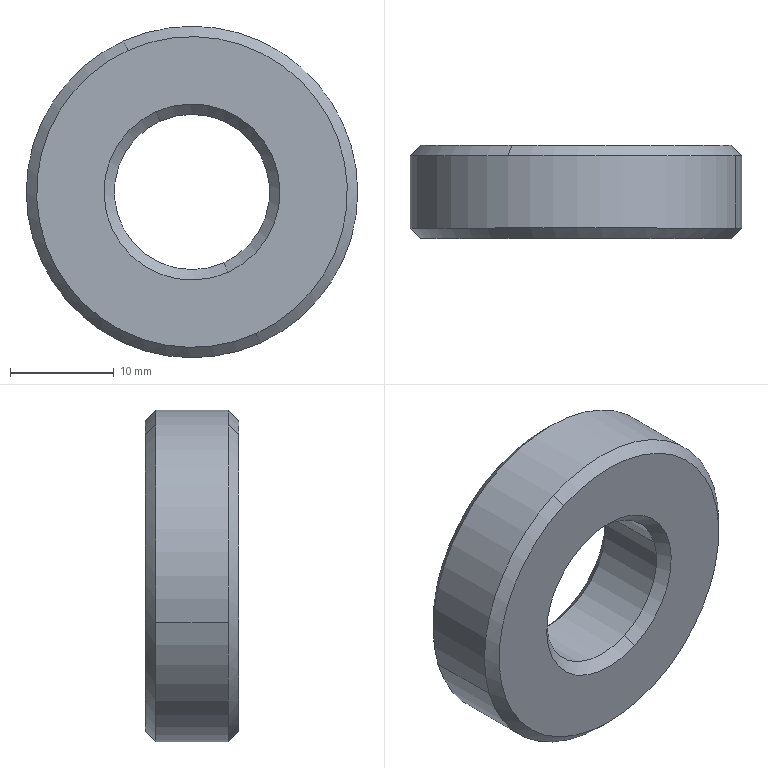Part | SolidWorks | features BaseBody 1 | 1 solid | 14 faces | box 32 x 9 x 32 mm | volume 5500 mm3 | cone 8 | cylinder 4 | plane 2 | commonest cylinder face diameters 15 x2 32 x2
STEP:
#1=CARTESIAN_POINT('',(-381.352,-113.,29.799));
#2=VERTEX_POINT('',#1);
#3=CARTESIAN_POINT('',(-393.697,-113.,57.141));
#4=VERTEX_POINT('',#3);
#5=CARTESIAN_POINT('',(-387.524,-113.,43.47));
#6=DIRECTION('',(0.,1.,0.));
#7=DIRECTION('',(-0.9598,0.,-0.2807));
#8=AXIS2_PLACEMENT_3D('',#5,#6,#7);
#9=CIRCLE('',#8,15.);
#10=EDGE_CURVE('',#2,#4,#9,.T.);
#11=ORIENTED_EDGE('',*,*,#10,.F.);
#12=CARTESIAN_POINT('',(-380.94,-114.,28.888));
#13=VERTEX_POINT('',#12);
#14=CARTESIAN_POINT('',(-381.146,-113.5,29.343));
#15=DIRECTION('',(0.291,-0.7071,-0.6445));
#16=VECTOR('',#15,1000.);
#17=LINE('',#14,#16);
#18=EDGE_CURVE('',#2,#13,#17,.T.);
#19=ORIENTED_EDGE('',*,*,#18,.T.);
#20=CARTESIAN_POINT('',(-402.881,-114.,38.979));
#21=VERTEX_POINT('',#20);
#22=CARTESIAN_POINT('',(-387.524,-114.,43.47));
#23=DIRECTION('',(0.,1.,0.));
#24=DIRECTION('',(-0.9598,0.,-0.2807));
#25=AXIS2_PLACEMENT_3D('',#22,#23,#24);
#26=CIRCLE('',#25,16.);
#27=EDGE_CURVE('',#13,#21,#26,.T.);
#28=ORIENTED_EDGE('',*,*,#27,.T.);
#29=CARTESIAN_POINT('',(-394.109,-114.,58.053));
#30=VERTEX_POINT('',#29);
#31=CARTESIAN_POINT('',(-387.524,-114.,43.47));
#32=DIRECTION('',(0.,1.,0.));
#33=DIRECTION('',(-0.9598,0.,-0.2807));
#34=AXIS2_PLACEMENT_3D('',#31,#32,#33);
#35=CIRCLE('',#34,16.);
#36=EDGE_CURVE('',#21,#30,#35,.T.);
#37=ORIENTED_EDGE('',*,*,#36,.T.);
#38=CARTESIAN_POINT('',(-393.903,-113.5,57.597));
#39=DIRECTION('',(-0.291,-0.7071,0.6445));
#40=VECTOR('',#39,1000.);
#41=LINE('',#38,#40);
#42=EDGE_CURVE('',#4,#30,#41,.T.);
#43=ORIENTED_EDGE('',*,*,#42,.F.);
#44=EDGE_LOOP('',(#11,#19,#28,#37,#43));
#45=FACE_OUTER_BOUND('',#44,.T.);
#46=CARTESIAN_POINT('',(-387.524,-113.5,43.47));
#47=DIRECTION('',(0.,-1.,0.));
#48=DIRECTION('',(-0.4115,0.,0.9114));
#49=AXIS2_PLACEMENT_3D('',#46,#47,#48);
#50=CONICAL_SURFACE('',#49,15.5,0.7854);
#51=ADVANCED_FACE('',(#45),#50,.T.);
#52=CARTESIAN_POINT('',(-381.352,-122.,29.799));
#53=VERTEX_POINT('',#52);
#54=CARTESIAN_POINT('',(-393.697,-122.,57.141));
#55=VERTEX_POINT('',#54);
#56=CARTESIAN_POINT('',(-387.524,-122.,43.47));
#57=DIRECTION('',(0.,-1.,0.));
#58=DIRECTION('',(0.9598,0.,0.2807));
#59=AXIS2_PLACEMENT_3D('',#56,#57,#58);
#60=CIRCLE('',#59,15.);
#61=EDGE_CURVE('',#53,#55,#60,.T.);
#62=ORIENTED_EDGE('',*,*,#61,.F.);
#63=CARTESIAN_POINT('',(-380.94,-121.,28.888));
#64=VERTEX_POINT('',#63);
#65=CARTESIAN_POINT('',(-381.146,-121.5,29.343));
#66=DIRECTION('',(0.291,0.7071,-0.6445));
#67=VECTOR('',#66,1000.);
#68=LINE('',#65,#67);
#69=EDGE_CURVE('',#53,#64,#68,.T.);
#70=ORIENTED_EDGE('',*,*,#69,.T.);
#71=CARTESIAN_POINT('',(-372.168,-121.,47.961));
#72=VERTEX_POINT('',#71);
#73=CARTESIAN_POINT('',(-387.524,-121.,43.47));
#74=DIRECTION('',(0.,-1.,0.));
#75=DIRECTION('',(0.9598,0.,0.2807));
#76=AXIS2_PLACEMENT_3D('',#73,#74,#75);
#77=CIRCLE('',#76,16.);
#78=EDGE_CURVE('',#64,#72,#77,.T.);
#79=ORIENTED_EDGE('',*,*,#78,.T.);
#80=CARTESIAN_POINT('',(-394.109,-121.,58.053));
#81=VERTEX_POINT('',#80);
#82=CARTESIAN_POINT('',(-387.524,-121.,43.47));
#83=DIRECTION('',(0.,-1.,0.));
#84=DIRECTION('',(0.9598,0.,0.2807));
#85=AXIS2_PLACEMENT_3D('',#82,#83,#84);
#86=CIRCLE('',#85,16.);
#87=EDGE_CURVE('',#72,#81,#86,.T.);
#88=ORIENTED_EDGE('',*,*,#87,.T.);
#89=CARTESIAN_POINT('',(-393.903,-121.5,57.597));
#90=DIRECTION('',(-0.291,0.7071,0.6445));
#91=VECTOR('',#90,1000.);
#92=LINE('',#89,#91);
#93=EDGE_CURVE('',#55,#81,#92,.T.);
#94=ORIENTED_EDGE('',*,*,#93,.F.);
#95=EDGE_LOOP('',(#62,#70,#79,#88,#94));
#96=FACE_OUTER_BOUND('',#95,.T.);
#97=CARTESIAN_POINT('',(-387.524,-121.5,43.47));
#98=DIRECTION('',(0.,1.,0.));
#99=DIRECTION('',(-0.4115,0.,0.9114));
#100=AXIS2_PLACEMENT_3D('',#97,#98,#99);
#101=CONICAL_SURFACE('',#100,15.5,0.7854);
#102=ADVANCED_FACE('',(#96),#101,.T.);
#103=CARTESIAN_POINT('',(-380.326,-121.,45.575));
#104=VERTEX_POINT('',#103);
#105=CARTESIAN_POINT('',(-384.438,-121.,36.635));
#106=VERTEX_POINT('',#105);
#107=CARTESIAN_POINT('',(-387.524,-121.,43.47));
#108=DIRECTION('',(0.,1.,0.));
#109=DIRECTION('',(-0.9598,0.,-0.2807));
#110=AXIS2_PLACEMENT_3D('',#107,#108,#109);
#111=CIRCLE('',#110,7.5);
#112=EDGE_CURVE('',#104,#106,#111,.T.);
#113=ORIENTED_EDGE('',*,*,#112,.T.);
#114=CARTESIAN_POINT('',(-384.027,-122.,35.723));
#115=VERTEX_POINT('',#114);
#116=CARTESIAN_POINT('',(-384.232,-121.5,36.179));
#117=DIRECTION('',(0.291,-0.7071,-0.6445));
#118=VECTOR('',#117,1000.);
#119=LINE('',#116,#118);
#120=EDGE_CURVE('',#106,#115,#119,.T.);
#121=ORIENTED_EDGE('',*,*,#120,.T.);
#122=CARTESIAN_POINT('',(-391.022,-122.,51.217));
#123=VERTEX_POINT('',#122);
#124=CARTESIAN_POINT('',(-387.524,-122.,43.47));
#125=DIRECTION('',(0.,1.,0.));
#126=DIRECTION('',(-0.9598,0.,-0.2807));
#127=AXIS2_PLACEMENT_3D('',#124,#125,#126);
#128=CIRCLE('',#127,8.5);
#129=EDGE_CURVE('',#123,#115,#128,.T.);
#130=ORIENTED_EDGE('',*,*,#129,.F.);
#131=CARTESIAN_POINT('',(-390.611,-121.,50.306));
#132=VERTEX_POINT('',#131);
#133=CARTESIAN_POINT('',(-390.817,-121.5,50.761));
#134=DIRECTION('',(-0.291,-0.7071,0.6445));
#135=VECTOR('',#134,1000.);
#136=LINE('',#133,#135);
#137=EDGE_CURVE('',#132,#123,#136,.T.);
#138=ORIENTED_EDGE('',*,*,#137,.F.);
#139=CARTESIAN_POINT('',(-387.524,-121.,43.47));
#140=DIRECTION('',(0.,1.,0.));
#141=DIRECTION('',(-0.9598,0.,-0.2807));
#142=AXIS2_PLACEMENT_3D('',#139,#140,#141);
#143=CIRCLE('',#142,7.5);
#144=EDGE_CURVE('',#132,#104,#143,.T.);
#145=ORIENTED_EDGE('',*,*,#144,.T.);
#146=EDGE_LOOP('',(#113,#121,#130,#138,#145));
#147=FACE_OUTER_BOUND('',#146,.T.);
#148=CARTESIAN_POINT('',(-387.524,-121.5,43.47));
#149=DIRECTION('',(0.,-1.,0.));
#150=DIRECTION('',(-0.4115,0.,0.9114));
#151=AXIS2_PLACEMENT_3D('',#148,#149,#150);
#152=CONICAL_SURFACE('',#151,8.,0.7854);
#153=ADVANCED_FACE('',(#147),#152,.F.);
#154=CARTESIAN_POINT('',(-394.723,-114.,41.365));
#155=VERTEX_POINT('',#154);
#156=CARTESIAN_POINT('',(-384.438,-114.,36.635));
#157=VERTEX_POINT('',#156);
#158=CARTESIAN_POINT('',(-387.524,-114.,43.47));
#159=DIRECTION('',(0.,-1.,0.));
#160=DIRECTION('',(0.9598,0.,0.2807));
#161=AXIS2_PLACEMENT_3D('',#158,#159,#160);
#162=CIRCLE('',#161,7.5);
#163=EDGE_CURVE('',#155,#157,#162,.T.);
#164=ORIENTED_EDGE('',*,*,#163,.T.);
#165=CARTESIAN_POINT('',(-384.027,-113.,35.723));
#166=VERTEX_POINT('',#165);
#167=CARTESIAN_POINT('',(-384.232,-113.5,36.179));
#168=DIRECTION('',(0.291,0.7071,-0.6445));
#169=VECTOR('',#168,1000.);
#170=LINE('',#167,#169);
#171=EDGE_CURVE('',#157,#166,#170,.T.);
#172=ORIENTED_EDGE('',*,*,#171,.T.);
#173=CARTESIAN_POINT('',(-391.022,-113.,51.217));
#174=VERTEX_POINT('',#173);
#175=CARTESIAN_POINT('',(-387.524,-113.,43.47));
#176=DIRECTION('',(0.,-1.,0.));
#177=DIRECTION('',(0.9598,0.,0.2807));
#178=AXIS2_PLACEMENT_3D('',#175,#176,#177);
#179=CIRCLE('',#178,8.5);
#180=EDGE_CURVE('',#174,#166,#179,.T.);
#181=ORIENTED_EDGE('',*,*,#180,.F.);
#182=CARTESIAN_POINT('',(-390.611,-114.,50.306));
#183=VERTEX_POINT('',#182);
#184=CARTESIAN_POINT('',(-390.817,-113.5,50.761));
#185=DIRECTION('',(-0.291,0.7071,0.6445));
#186=VECTOR('',#185,1000.);
#187=LINE('',#184,#186);
#188=EDGE_CURVE('',#183,#174,#187,.T.);
#189=ORIENTED_EDGE('',*,*,#188,.F.);
#190=CARTESIAN_POINT('',(-387.524,-114.,43.47));
#191=DIRECTION('',(0.,-1.,0.));
#192=DIRECTION('',(0.9598,0.,0.2807));
#193=AXIS2_PLACEMENT_3D('',#190,#191,#192);
#194=CIRCLE('',#193,7.5);
#195=EDGE_CURVE('',#183,#155,#194,.T.);
#196=ORIENTED_EDGE('',*,*,#195,.T.);
#197=EDGE_LOOP('',(#164,#172,#181,#189,#196));
#198=FACE_OUTER_BOUND('',#197,.T.);
#199=CARTESIAN_POINT('',(-387.524,-113.5,43.47));
#200=DIRECTION('',(0.,1.,0.));
#201=DIRECTION('',(-0.4115,0.,0.9114));
#202=AXIS2_PLACEMENT_3D('',#199,#200,#201);
#203=CONICAL_SURFACE('',#202,8.,0.7854);
#204=ADVANCED_FACE('',(#198),#203,.F.);
#205=ORIENTED_EDGE('',*,*,#163,.F.);
#206=CARTESIAN_POINT('',(-394.723,-121.,41.365));
#207=VERTEX_POINT('',#206);
#208=CARTESIAN_POINT('',(-394.723,-113.,41.365));
#209=DIRECTION('',(0.,-1.,0.));
#210=VECTOR('',#209,1000.);
#211=LINE('',#208,#210);
#212=EDGE_CURVE('',#155,#207,#211,.T.);
#213=ORIENTED_EDGE('',*,*,#212,.T.);
#214=CARTESIAN_POINT('',(-387.524,-121.,43.47));
#215=DIRECTION('',(0.,1.,0.));
#216=DIRECTION('',(-0.9598,0.,-0.2807));
#217=AXIS2_PLACEMENT_3D('',#214,#215,#216);
#218=CIRCLE('',#217,7.5);
#219=EDGE_CURVE('',#106,#207,#218,.T.);
#220=ORIENTED_EDGE('',*,*,#219,.F.);
#221=ORIENTED_EDGE('',*,*,#112,.F.);
#222=CARTESIAN_POINT('',(-380.326,-114.,45.575));
#223=VERTEX_POINT('',#222);
#224=CARTESIAN_POINT('',(-380.326,-113.,45.575));
#225=DIRECTION('',(0.,-1.,0.));
#226=VECTOR('',#225,1000.);
#227=LINE('',#224,#226);
#228=EDGE_CURVE('',#223,#104,#227,.T.);
#229=ORIENTED_EDGE('',*,*,#228,.F.);
#230=CARTESIAN_POINT('',(-387.524,-114.,43.47));
#231=DIRECTION('',(0.,-1.,0.));
#232=DIRECTION('',(0.9598,0.,0.2807));
#233=AXIS2_PLACEMENT_3D('',#230,#231,#232);
#234=CIRCLE('',#233,7.5);
#235=EDGE_CURVE('',#157,#223,#234,.T.);
#236=ORIENTED_EDGE('',*,*,#235,.F.);
#237=EDGE_LOOP('',(#205,#213,#220,#221,#229,#236));
#238=FACE_OUTER_BOUND('',#237,.T.);
#239=CARTESIAN_POINT('',(-387.524,-113.,43.47));
#240=DIRECTION('',(0.,-1.,0.));
#241=DIRECTION('',(0.9598,0.,0.2807));
#242=AXIS2_PLACEMENT_3D('',#239,#240,#241);
#243=CYLINDRICAL_SURFACE('',#242,7.5);
#244=ADVANCED_FACE('',(#238),#243,.F.);
#245=ORIENTED_EDGE('',*,*,#36,.F.);
#246=CARTESIAN_POINT('',(-402.881,-121.,38.979));
#247=VERTEX_POINT('',#246);
#248=CARTESIAN_POINT('',(-402.881,-113.,38.979));
#249=DIRECTION('',(0.,-1.,0.));
#250=VECTOR('',#249,1000.);
#251=LINE('',#248,#250);
#252=EDGE_CURVE('',#21,#247,#251,.T.);
#253=ORIENTED_EDGE('',*,*,#252,.T.);
#254=CARTESIAN_POINT('',(-387.524,-121.,43.47));
#255=DIRECTION('',(0.,-1.,0.));
#256=DIRECTION('',(0.9598,0.,0.2807));
#257=AXIS2_PLACEMENT_3D('',#254,#255,#256);
#258=CIRCLE('',#257,16.);
#259=EDGE_CURVE('',#81,#247,#258,.T.);
#260=ORIENTED_EDGE('',*,*,#259,.F.);
#261=ORIENTED_EDGE('',*,*,#87,.F.);
#262=CARTESIAN_POINT('',(-372.168,-114.,47.961));
#263=VERTEX_POINT('',#262);
#264=CARTESIAN_POINT('',(-372.168,-113.,47.961));
#265=DIRECTION('',(0.,-1.,0.));
#266=VECTOR('',#265,1000.);
#267=LINE('',#264,#266);
#268=EDGE_CURVE('',#263,#72,#267,.T.);
#269=ORIENTED_EDGE('',*,*,#268,.F.);
#270=CARTESIAN_POINT('',(-387.524,-114.,43.47));
#271=DIRECTION('',(0.,1.,0.));
#272=DIRECTION('',(-0.9598,0.,-0.2807));
#273=AXIS2_PLACEMENT_3D('',#270,#271,#272);
#274=CIRCLE('',#273,16.);
#275=EDGE_CURVE('',#30,#263,#274,.T.);
#276=ORIENTED_EDGE('',*,*,#275,.F.);
#277=EDGE_LOOP('',(#245,#253,#260,#261,#269,#276));
#278=FACE_OUTER_BOUND('',#277,.T.);
#279=CARTESIAN_POINT('',(-387.524,-113.,43.47));
#280=DIRECTION('',(0.,-1.,0.));
#281=DIRECTION('',(0.9598,0.,0.2807));
#282=AXIS2_PLACEMENT_3D('',#279,#280,#281);
#283=CYLINDRICAL_SURFACE('',#282,16.);
#284=ADVANCED_FACE('',(#278),#283,.T.);
#285=ORIENTED_EDGE('',*,*,#180,.T.);
#286=CARTESIAN_POINT('',(-387.524,-113.,43.47));
#287=DIRECTION('',(0.,-1.,0.));
#288=DIRECTION('',(0.9598,0.,0.2807));
#289=AXIS2_PLACEMENT_3D('',#286,#287,#288);
#290=CIRCLE('',#289,8.5);
#291=EDGE_CURVE('',#166,#174,#290,.T.);
#292=ORIENTED_EDGE('',*,*,#291,.T.);
#293=EDGE_LOOP('',(#285,#292));
#294=FACE_BOUND('',#293,.T.);
#295=CARTESIAN_POINT('',(-387.524,-113.,43.47));
#296=DIRECTION('',(0.,1.,0.));
#297=DIRECTION('',(-0.9598,0.,-0.2807));
#298=AXIS2_PLACEMENT_3D('',#295,#296,#297);
#299=CIRCLE('',#298,15.);
#300=EDGE_CURVE('',#4,#2,#299,.T.);
#301=ORIENTED_EDGE('',*,*,#300,.T.);
#302=ORIENTED_EDGE('',*,*,#10,.T.);
#303=EDGE_LOOP('',(#301,#302));
#304=FACE_OUTER_BOUND('',#303,.T.);
#305=CARTESIAN_POINT('',(-402.493,-113.,22.962));
#306=DIRECTION('',(0.,-1.,0.));
#307=DIRECTION('',(0.,0.,-1.));
#308=AXIS2_PLACEMENT_3D('',#305,#306,#307);
#309=PLANE('',#308);
#310=ADVANCED_FACE('',(#294,#304),#309,.F.);
#311=ORIENTED_EDGE('',*,*,#129,.T.);
#312=CARTESIAN_POINT('',(-387.524,-122.,43.47));
#313=DIRECTION('',(0.,1.,0.));
#314=DIRECTION('',(-0.9598,0.,-0.2807));
#315=AXIS2_PLACEMENT_3D('',#312,#313,#314);
#316=CIRCLE('',#315,8.5);
#317=EDGE_CURVE('',#115,#123,#316,.T.);
#318=ORIENTED_EDGE('',*,*,#317,.T.);
#319=EDGE_LOOP('',(#311,#318));
#320=FACE_BOUND('',#319,.T.);
#321=CARTESIAN_POINT('',(-387.524,-122.,43.47));
#322=DIRECTION('',(0.,-1.,0.));
#323=DIRECTION('',(0.9598,0.,0.2807));
#324=AXIS2_PLACEMENT_3D('',#321,#322,#323);
#325=CIRCLE('',#324,15.);
#326=EDGE_CURVE('',#55,#53,#325,.T.);
#327=ORIENTED_EDGE('',*,*,#326,.T.);
#328=ORIENTED_EDGE('',*,*,#61,.T.);
#329=EDGE_LOOP('',(#327,#328));
#330=FACE_OUTER_BOUND('',#329,.T.);
#331=CARTESIAN_POINT('',(-402.493,-122.,22.962));
#332=DIRECTION('',(0.,-1.,0.));
#333=DIRECTION('',(0.,0.,-1.));
#334=AXIS2_PLACEMENT_3D('',#331,#332,#333);
#335=PLANE('',#334);
#336=ADVANCED_FACE('',(#320,#330),#335,.T.);
#337=ORIENTED_EDGE('',*,*,#252,.F.);
#338=ORIENTED_EDGE('',*,*,#27,.F.);
#339=CARTESIAN_POINT('',(-387.524,-114.,43.47));
#340=DIRECTION('',(0.,1.,0.));
#341=DIRECTION('',(-0.9598,0.,-0.2807));
#342=AXIS2_PLACEMENT_3D('',#339,#340,#341);
#343=CIRCLE('',#342,16.);
#344=EDGE_CURVE('',#263,#13,#343,.T.);
#345=ORIENTED_EDGE('',*,*,#344,.F.);
#346=ORIENTED_EDGE('',*,*,#268,.T.);
#347=ORIENTED_EDGE('',*,*,#78,.F.);
#348=CARTESIAN_POINT('',(-387.524,-121.,43.47));
#349=DIRECTION('',(0.,-1.,0.));
#350=DIRECTION('',(0.9598,0.,0.2807));
#351=AXIS2_PLACEMENT_3D('',#348,#349,#350);
#352=CIRCLE('',#351,16.);
#353=EDGE_CURVE('',#247,#64,#352,.T.);
#354=ORIENTED_EDGE('',*,*,#353,.F.);
#355=EDGE_LOOP('',(#337,#338,#345,#346,#347,#354));
#356=FACE_OUTER_BOUND('',#355,.T.);
#357=CARTESIAN_POINT('',(-387.524,-113.,43.47));
#358=DIRECTION('',(0.,-1.,0.));
#359=DIRECTION('',(0.9598,0.,0.2807));
#360=AXIS2_PLACEMENT_3D('',#357,#358,#359);
#361=CYLINDRICAL_SURFACE('',#360,16.);
#362=ADVANCED_FACE('',(#356),#361,.T.);
#363=ORIENTED_EDGE('',*,*,#212,.F.);
#364=ORIENTED_EDGE('',*,*,#195,.F.);
#365=CARTESIAN_POINT('',(-387.524,-114.,43.47));
#366=DIRECTION('',(0.,-1.,0.));
#367=DIRECTION('',(0.9598,0.,0.2807));
#368=AXIS2_PLACEMENT_3D('',#365,#366,#367);
#369=CIRCLE('',#368,7.5);
#370=EDGE_CURVE('',#223,#183,#369,.T.);
#371=ORIENTED_EDGE('',*,*,#370,.F.);
#372=ORIENTED_EDGE('',*,*,#228,.T.);
#373=ORIENTED_EDGE('',*,*,#144,.F.);
#374=CARTESIAN_POINT('',(-387.524,-121.,43.47));
#375=DIRECTION('',(0.,1.,0.));
#376=DIRECTION('',(-0.9598,0.,-0.2807));
#377=AXIS2_PLACEMENT_3D('',#374,#375,#376);
#378=CIRCLE('',#377,7.5);
#379=EDGE_CURVE('',#207,#132,#378,.T.);
#380=ORIENTED_EDGE('',*,*,#379,.F.);
#381=EDGE_LOOP('',(#363,#364,#371,#372,#373,#380));
#382=FACE_OUTER_BOUND('',#381,.T.);
#383=CARTESIAN_POINT('',(-387.524,-113.,43.47));
#384=DIRECTION('',(0.,-1.,0.));
#385=DIRECTION('',(0.9598,0.,0.2807));
#386=AXIS2_PLACEMENT_3D('',#383,#384,#385);
#387=CYLINDRICAL_SURFACE('',#386,7.5);
#388=ADVANCED_FACE('',(#382),#387,.F.);
#389=ORIENTED_EDGE('',*,*,#171,.F.);
#390=ORIENTED_EDGE('',*,*,#235,.T.);
#391=ORIENTED_EDGE('',*,*,#370,.T.);
#392=ORIENTED_EDGE('',*,*,#188,.T.);
#393=ORIENTED_EDGE('',*,*,#291,.F.);
#394=EDGE_LOOP('',(#389,#390,#391,#392,#393));
#395=FACE_OUTER_BOUND('',#394,.T.);
#396=CARTESIAN_POINT('',(-387.524,-113.5,43.47));
#397=DIRECTION('',(0.,1.,0.));
#398=DIRECTION('',(-0.4115,0.,0.9114));
#399=AXIS2_PLACEMENT_3D('',#396,#397,#398);
#400=CONICAL_SURFACE('',#399,8.,0.7854);
#401=ADVANCED_FACE('',(#395),#400,.F.);
#402=ORIENTED_EDGE('',*,*,#120,.F.);
#403=ORIENTED_EDGE('',*,*,#219,.T.);
#404=ORIENTED_EDGE('',*,*,#379,.T.);
#405=ORIENTED_EDGE('',*,*,#137,.T.);
#406=ORIENTED_EDGE('',*,*,#317,.F.);
#407=EDGE_LOOP('',(#402,#403,#404,#405,#406));
#408=FACE_OUTER_BOUND('',#407,.T.);
#409=CARTESIAN_POINT('',(-387.524,-121.5,43.47));
#410=DIRECTION('',(0.,-1.,0.));
#411=DIRECTION('',(-0.4115,0.,0.9114));
#412=AXIS2_PLACEMENT_3D('',#409,#410,#411);
#413=CONICAL_SURFACE('',#412,8.,0.7854);
#414=ADVANCED_FACE('',(#408),#413,.F.);
#415=ORIENTED_EDGE('',*,*,#69,.F.);
#416=ORIENTED_EDGE('',*,*,#326,.F.);
#417=ORIENTED_EDGE('',*,*,#93,.T.);
#418=ORIENTED_EDGE('',*,*,#259,.T.);
#419=ORIENTED_EDGE('',*,*,#353,.T.);
#420=EDGE_LOOP('',(#415,#416,#417,#418,#419));
#421=FACE_OUTER_BOUND('',#420,.T.);
#422=CARTESIAN_POINT('',(-387.524,-121.5,43.47));
#423=DIRECTION('',(0.,1.,0.));
#424=DIRECTION('',(-0.4115,0.,0.9114));
#425=AXIS2_PLACEMENT_3D('',#422,#423,#424);
#426=CONICAL_SURFACE('',#425,15.5,0.7854);
#427=ADVANCED_FACE('',(#421),#426,.T.);
#428=ORIENTED_EDGE('',*,*,#18,.F.);
#429=ORIENTED_EDGE('',*,*,#300,.F.);
#430=ORIENTED_EDGE('',*,*,#42,.T.);
#431=ORIENTED_EDGE('',*,*,#275,.T.);
#432=ORIENTED_EDGE('',*,*,#344,.T.);
#433=EDGE_LOOP('',(#428,#429,#430,#431,#432));
#434=FACE_OUTER_BOUND('',#433,.T.);
#435=CARTESIAN_POINT('',(-387.524,-113.5,43.47));
#436=DIRECTION('',(0.,-1.,0.));
#437=DIRECTION('',(-0.4115,0.,0.9114));
#438=AXIS2_PLACEMENT_3D('',#435,#436,#437);
#439=CONICAL_SURFACE('',#438,15.5,0.7854);
#440=ADVANCED_FACE('',(#434),#439,.T.);
#441=CLOSED_SHELL('',(#51,#102,#153,#204,#244,#284,#310,#336,#362,#388,#401,#414,#427,#440));
#442=MANIFOLD_SOLID_BREP('',#441);
#443=CARTESIAN_POINT('',(0.,0.,0.));
#444=DIRECTION('',(0.,0.,1.));
#445=DIRECTION('',(1.,0.,0.));
#446=AXIS2_PLACEMENT_3D('',#443,#444,#445);
#447=(LENGTH_UNIT()NAMED_UNIT(*)SI_UNIT(.MILLI.,.METRE.));
#448=UNCERTAINTY_MEASURE_WITH_UNIT(LENGTH_MEASURE(0.00001),#447,'','');
#449=(NAMED_UNIT(*)PLANE_ANGLE_UNIT()SI_UNIT($,.RADIAN.));
#450=(NAMED_UNIT(*)SI_UNIT($,.STERADIAN.)SOLID_ANGLE_UNIT());
#451=(GEOMETRIC_REPRESENTATION_CONTEXT(3)GLOBAL_UNCERTAINTY_ASSIGNED_CONTEXT((#448))GLOBAL_UNIT_ASSIGNED_CONTEXT((#447,#449,#450))REPRESENTATION_CONTEXT('',''));
#452=ADVANCED_BREP_SHAPE_REPRESENTATION('',(#442,#446),#451);